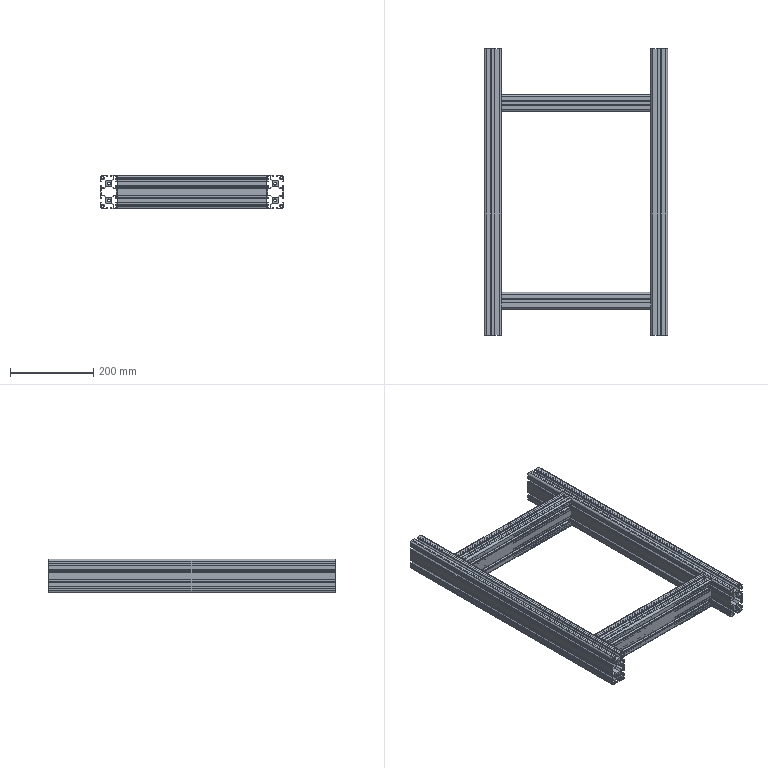Part | STEP file | PN_0014_default<as machined> | 4 solids | 617 faces | box 439.002 x 686.5 x 80 mm | volume 2058365 mm3 | plane 568 | cylinder 49 | commonest cylinder face diameters 9 x17 5 x16 6.8 x16